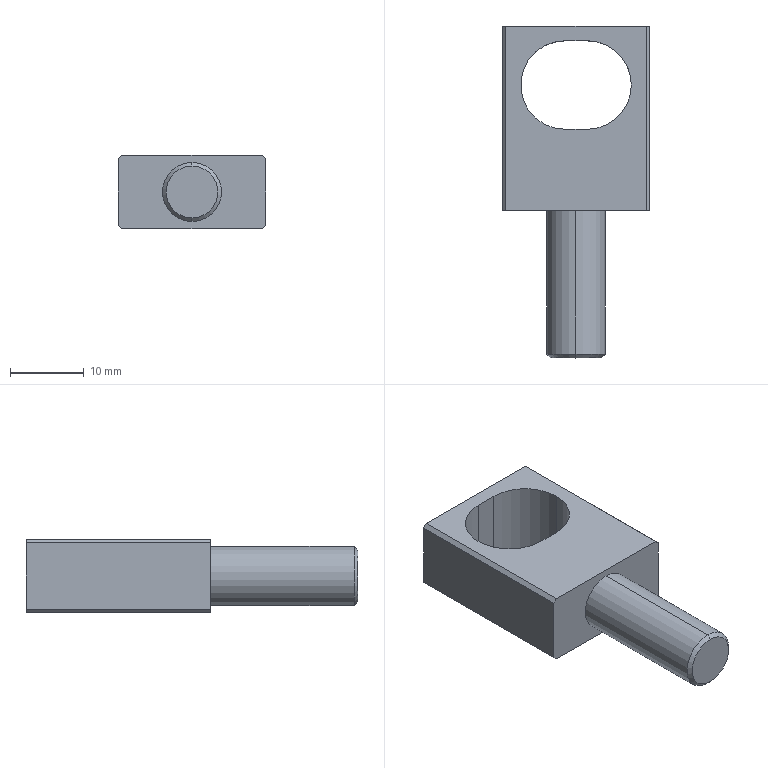Part | STEP file | 8ZY.143.1010 | 1 solid | 20 faces | box 20 x 45 x 10 mm | volume 4499 mm3 | plane 13 | cylinder 5 | cone 2 | commonest cylinder face diameters 12 x3 8 x2
STEP:
#1=CARTESIAN_POINT('',(0.,0.,0.));
#2=DIRECTION('',(0.,0.,1.));
#3=DIRECTION('',(1.,0.,0.));
#4=AXIS2_PLACEMENT_3D('',#1,#2,#3);
#5=CARTESIAN_POINT('',(1.5,10.5,-10.));
#6=VERTEX_POINT('',#5);
#7=CARTESIAN_POINT('',(1.5,10.5,0.));
#8=VERTEX_POINT('',#7);
#9=CARTESIAN_POINT('',(1.5,10.5,-10.));
#10=DIRECTION('',(0.,0.,1.));
#11=VECTOR('',#10,1.);
#12=LINE('',#9,#11);
#13=CARTESIAN_POINT('',(1.5,4.5,-10.));
#14=DIRECTION('',(0.,0.,1.));
#15=DIRECTION('',(1.,0.,0.));
#16=AXIS2_PLACEMENT_3D('',#13,#14,#15);
#17=CYLINDRICAL_SURFACE('',#16,6.);
#18=CARTESIAN_POINT('',(1.571,0.));
#19=DIRECTION('',(0.,1.));
#20=VECTOR('',#19,1.);
#21=LINE('',#18,#20);
#22=(GEOMETRIC_REPRESENTATION_CONTEXT(2)PARAMETRIC_REPRESENTATION_CONTEXT()REPRESENTATION_CONTEXT('',''));
#23=DEFINITIONAL_REPRESENTATION('',(#21),#22);
#24=PCURVE('',#17,#23);
#25=CARTESIAN_POINT('',(-1.5,10.5,-10.));
#26=DIRECTION('',(0.,1.,0.));
#27=DIRECTION('',(0.,0.,1.));
#28=AXIS2_PLACEMENT_3D('',#25,#26,#27);
#29=PLANE('',#28);
#30=CARTESIAN_POINT('',(0.,3.));
#31=DIRECTION('',(1.,0.));
#32=VECTOR('',#31,1.);
#33=LINE('',#30,#32);
#34=(GEOMETRIC_REPRESENTATION_CONTEXT(2)PARAMETRIC_REPRESENTATION_CONTEXT()REPRESENTATION_CONTEXT('',''));
#35=DEFINITIONAL_REPRESENTATION('',(#33),#34);
#36=PCURVE('',#29,#35);
#37=SURFACE_CURVE('',#12,(#24,#36),.PCURVE_S1.);
#38=EDGE_CURVE('',#6,#8,#37,.T.);
#39=ORIENTED_EDGE('',*,*,#38,.T.);
#40=CARTESIAN_POINT('',(7.5,4.5,0.));
#41=VERTEX_POINT('',#40);
#42=CARTESIAN_POINT('',(1.5,4.5,0.));
#43=DIRECTION('',(0.,0.,1.));
#44=DIRECTION('',(1.,0.,0.));
#45=AXIS2_PLACEMENT_3D('',#42,#43,#44);
#46=CIRCLE('',#45,6.);
#47=CARTESIAN_POINT('',(0.,10.));
#48=DIRECTION('',(1.,0.));
#49=VECTOR('',#48,1.);
#50=LINE('',#47,#49);
#51=(GEOMETRIC_REPRESENTATION_CONTEXT(2)PARAMETRIC_REPRESENTATION_CONTEXT()REPRESENTATION_CONTEXT('',''));
#52=DEFINITIONAL_REPRESENTATION('',(#50),#51);
#53=PCURVE('',#17,#52);
#54=CARTESIAN_POINT('',(-10.,-12.5,0.));
#55=DIRECTION('',(0.,0.,-1.));
#56=DIRECTION('',(-1.,0.,0.));
#57=AXIS2_PLACEMENT_3D('',#54,#55,#56);
#58=PLANE('',#57);
#59=CARTESIAN_POINT('',(-17.5,17.));
#60=CARTESIAN_POINT('',(-17.5,27.392));
#61=CARTESIAN_POINT('',(-8.5,22.196));
#62=CARTESIAN_POINT('',(0.5,17.));
#63=CARTESIAN_POINT('',(-8.5,11.804));
#64=CARTESIAN_POINT('',(-17.5,6.608));
#65=CARTESIAN_POINT('',(-17.5,17.));
#66=(BOUNDED_CURVE()B_SPLINE_CURVE(2,(#59,#60,#61,#62,#63,#64,#65),.UNSPECIFIED.,.T.,.F.)B_SPLINE_CURVE_WITH_KNOTS((1,2,2,2,2,1),(-2.094,0.,2.094,4.189,6.283,8.378),.UNSPECIFIED.)CURVE()GEOMETRIC_REPRESENTATION_ITEM()RATIONAL_B_SPLINE_CURVE((1.,0.5,1.,0.5,1.,0.5,1.))REPRESENTATION_ITEM(''));
#67=(GEOMETRIC_REPRESENTATION_CONTEXT(2)PARAMETRIC_REPRESENTATION_CONTEXT()REPRESENTATION_CONTEXT('',''));
#68=DEFINITIONAL_REPRESENTATION('',(#66),#67);
#69=PCURVE('',#58,#68);
#70=SURFACE_CURVE('',#46,(#53,#69),.PCURVE_S1.);
#71=EDGE_CURVE('',#41,#8,#70,.T.);
#72=ORIENTED_EDGE('',*,*,#71,.F.);
#73=CARTESIAN_POINT('',(7.5,4.5,-10.));
#74=VERTEX_POINT('',#73);
#75=CARTESIAN_POINT('',(7.5,4.5,-10.));
#76=DIRECTION('',(0.,0.,1.));
#77=VECTOR('',#76,1.);
#78=LINE('',#75,#77);
#79=CARTESIAN_POINT('',(0.,0.));
#80=DIRECTION('',(0.,1.));
#81=VECTOR('',#80,1.);
#82=LINE('',#79,#81);
#83=(GEOMETRIC_REPRESENTATION_CONTEXT(2)PARAMETRIC_REPRESENTATION_CONTEXT()REPRESENTATION_CONTEXT('',''));
#84=DEFINITIONAL_REPRESENTATION('',(#82),#83);
#85=PCURVE('',#17,#84);
#86=CARTESIAN_POINT('',(1.5,4.5,-10.));
#87=DIRECTION('',(0.,0.,1.));
#88=DIRECTION('',(1.,0.,0.));
#89=AXIS2_PLACEMENT_3D('',#86,#87,#88);
#90=CYLINDRICAL_SURFACE('',#89,6.);
#91=CARTESIAN_POINT('',(6.283,0.));
#92=DIRECTION('',(0.,1.));
#93=VECTOR('',#92,1.);
#94=LINE('',#91,#93);
#95=(GEOMETRIC_REPRESENTATION_CONTEXT(2)PARAMETRIC_REPRESENTATION_CONTEXT()REPRESENTATION_CONTEXT('',''));
#96=DEFINITIONAL_REPRESENTATION('',(#94),#95);
#97=PCURVE('',#90,#96);
#98=SURFACE_CURVE('',#78,(#85,#97),.PCURVE_S1.);
#99=EDGE_CURVE('',#74,#41,#98,.T.);
#100=ORIENTED_EDGE('',*,*,#99,.F.);
#101=CARTESIAN_POINT('',(1.5,4.5,-10.));
#102=DIRECTION('',(0.,0.,1.));
#103=DIRECTION('',(1.,0.,0.));
#104=AXIS2_PLACEMENT_3D('',#101,#102,#103);
#105=CIRCLE('',#104,6.);
#106=CARTESIAN_POINT('',(0.,0.));
#107=DIRECTION('',(1.,0.));
#108=VECTOR('',#107,1.);
#109=LINE('',#106,#108);
#110=(GEOMETRIC_REPRESENTATION_CONTEXT(2)PARAMETRIC_REPRESENTATION_CONTEXT()REPRESENTATION_CONTEXT('',''));
#111=DEFINITIONAL_REPRESENTATION('',(#109),#110);
#112=PCURVE('',#17,#111);
#113=CARTESIAN_POINT('',(-10.,-12.5,-10.));
#114=DIRECTION('',(0.,0.,-1.));
#115=DIRECTION('',(-1.,0.,0.));
#116=AXIS2_PLACEMENT_3D('',#113,#114,#115);
#117=PLANE('',#116);
#118=CARTESIAN_POINT('',(-17.5,17.));
#119=CARTESIAN_POINT('',(-17.5,27.392));
#120=CARTESIAN_POINT('',(-8.5,22.196));
#121=CARTESIAN_POINT('',(0.5,17.));
#122=CARTESIAN_POINT('',(-8.5,11.804));
#123=CARTESIAN_POINT('',(-17.5,6.608));
#124=CARTESIAN_POINT('',(-17.5,17.));
#125=(BOUNDED_CURVE()B_SPLINE_CURVE(2,(#118,#119,#120,#121,#122,#123,#124),.UNSPECIFIED.,.T.,.F.)B_SPLINE_CURVE_WITH_KNOTS((1,2,2,2,2,1),(-2.094,0.,2.094,4.189,6.283,8.378),.UNSPECIFIED.)CURVE()GEOMETRIC_REPRESENTATION_ITEM()RATIONAL_B_SPLINE_CURVE((1.,0.5,1.,0.5,1.,0.5,1.))REPRESENTATION_ITEM(''));
#126=(GEOMETRIC_REPRESENTATION_CONTEXT(2)PARAMETRIC_REPRESENTATION_CONTEXT()REPRESENTATION_CONTEXT('',''));
#127=DEFINITIONAL_REPRESENTATION('',(#125),#126);
#128=PCURVE('',#117,#127);
#129=SURFACE_CURVE('',#105,(#112,#128),.PCURVE_S1.);
#130=EDGE_CURVE('',#74,#6,#129,.T.);
#131=ORIENTED_EDGE('',*,*,#130,.T.);
#132=EDGE_LOOP('',(#39,#72,#100,#131));
#133=FACE_BOUND('',#132,.F.);
#134=ADVANCED_FACE('',(#133),#17,.F.);
#135=CARTESIAN_POINT('',(0.,-32.5,-8.5));
#136=VERTEX_POINT('',#135);
#137=CARTESIAN_POINT('',(0.,-32.5,-1.5));
#138=VERTEX_POINT('',#137);
#139=CARTESIAN_POINT('',(0.,-32.5,-5.));
#140=DIRECTION('',(0.,-1.,0.));
#141=DIRECTION('',(0.,0.,-1.));
#142=AXIS2_PLACEMENT_3D('',#139,#140,#141);
#143=CIRCLE('',#142,3.5);
#144=CARTESIAN_POINT('',(0.,-32.5,-5.));
#145=DIRECTION('',(0.,1.,0.));
#146=DIRECTION('',(0.,0.,1.));
#147=AXIS2_PLACEMENT_3D('',#144,#145,#146);
#148=CONICAL_SURFACE('',#147,3.5,0.7854);
#149=CARTESIAN_POINT('',(3.142,0.));
#150=DIRECTION('',(-1.,0.));
#151=VECTOR('',#150,1.);
#152=LINE('',#149,#151);
#153=(GEOMETRIC_REPRESENTATION_CONTEXT(2)PARAMETRIC_REPRESENTATION_CONTEXT()REPRESENTATION_CONTEXT('',''));
#154=DEFINITIONAL_REPRESENTATION('',(#152),#153);
#155=PCURVE('',#148,#154);
#156=CARTESIAN_POINT('',(0.,-32.5,-5.));
#157=DIRECTION('',(0.,-1.,0.));
#158=DIRECTION('',(0.,0.,-1.));
#159=AXIS2_PLACEMENT_3D('',#156,#157,#158);
#160=PLANE('',#159);
#161=CARTESIAN_POINT('',(0.,0.));
#162=DIRECTION('',(1.,0.));
#163=AXIS2_PLACEMENT_2D('',#161,#162);
#164=CIRCLE('',#163,3.5);
#165=(GEOMETRIC_REPRESENTATION_CONTEXT(2)PARAMETRIC_REPRESENTATION_CONTEXT()REPRESENTATION_CONTEXT('',''));
#166=DEFINITIONAL_REPRESENTATION('',(#164),#165);
#167=PCURVE('',#160,#166);
#168=SURFACE_CURVE('',#143,(#155,#167),.PCURVE_S1.);
#169=EDGE_CURVE('',#136,#138,#168,.T.);
#170=ORIENTED_EDGE('',*,*,#169,.F.);
#171=CARTESIAN_POINT('',(0.,-32.,-9.));
#172=VERTEX_POINT('',#171);
#173=CARTESIAN_POINT('',(0.,-32.5,-8.5));
#174=DIRECTION('',(0.,0.7071,-0.7071));
#175=VECTOR('',#174,1.);
#176=LINE('',#173,#175);
#177=CARTESIAN_POINT('',(3.142,0.));
#178=DIRECTION('',(0.,1.));
#179=VECTOR('',#178,1.);
#180=LINE('',#177,#179);
#181=(GEOMETRIC_REPRESENTATION_CONTEXT(2)PARAMETRIC_REPRESENTATION_CONTEXT()REPRESENTATION_CONTEXT('',''));
#182=DEFINITIONAL_REPRESENTATION('',(#180),#181);
#183=PCURVE('',#148,#182);
#184=CARTESIAN_POINT('',(0.,-32.5,-5.));
#185=DIRECTION('',(0.,1.,0.));
#186=DIRECTION('',(0.,0.,1.));
#187=AXIS2_PLACEMENT_3D('',#184,#185,#186);
#188=CONICAL_SURFACE('',#187,3.5,0.7854);
#189=CARTESIAN_POINT('',(3.142,0.));
#190=DIRECTION('',(0.,1.));
#191=VECTOR('',#190,1.);
#192=LINE('',#189,#191);
#193=(GEOMETRIC_REPRESENTATION_CONTEXT(2)PARAMETRIC_REPRESENTATION_CONTEXT()REPRESENTATION_CONTEXT('',''));
#194=DEFINITIONAL_REPRESENTATION('',(#192),#193);
#195=PCURVE('',#188,#194);
#196=SURFACE_CURVE('',#176,(#183,#195),.PCURVE_S1.);
#197=EDGE_CURVE('',#136,#172,#196,.T.);
#198=ORIENTED_EDGE('',*,*,#197,.T.);
#199=CARTESIAN_POINT('',(0.,-32.,-1.));
#200=VERTEX_POINT('',#199);
#201=CARTESIAN_POINT('',(0.,-32.,-5.));
#202=DIRECTION('',(0.,1.,0.));
#203=DIRECTION('',(0.,0.,-1.));
#204=AXIS2_PLACEMENT_3D('',#201,#202,#203);
#205=CIRCLE('',#204,4.);
#206=CARTESIAN_POINT('',(-3.142,0.5));
#207=DIRECTION('',(1.,0.));
#208=VECTOR('',#207,1.);
#209=LINE('',#206,#208);
#210=(GEOMETRIC_REPRESENTATION_CONTEXT(2)PARAMETRIC_REPRESENTATION_CONTEXT()REPRESENTATION_CONTEXT('',''));
#211=DEFINITIONAL_REPRESENTATION('',(#209),#210);
#212=PCURVE('',#148,#211);
#213=CARTESIAN_POINT('',(0.,-32.5,-5.));
#214=DIRECTION('',(0.,1.,0.));
#215=DIRECTION('',(0.,0.,1.));
#216=AXIS2_PLACEMENT_3D('',#213,#214,#215);
#217=CYLINDRICAL_SURFACE('',#216,4.);
#218=CARTESIAN_POINT('',(-3.142,0.5));
#219=DIRECTION('',(1.,0.));
#220=VECTOR('',#219,1.);
#221=LINE('',#218,#220);
#222=(GEOMETRIC_REPRESENTATION_CONTEXT(2)PARAMETRIC_REPRESENTATION_CONTEXT()REPRESENTATION_CONTEXT('',''));
#223=DEFINITIONAL_REPRESENTATION('',(#221),#222);
#224=PCURVE('',#217,#223);
#225=SURFACE_CURVE('',#205,(#212,#224),.PCURVE_S1.);
#226=EDGE_CURVE('',#200,#172,#225,.T.);
#227=ORIENTED_EDGE('',*,*,#226,.F.);
#228=CARTESIAN_POINT('',(0.,-32.5,-1.5));
#229=DIRECTION('',(0.,0.7071,0.7071));
#230=VECTOR('',#229,1.);
#231=LINE('',#228,#230);
#232=CARTESIAN_POINT('',(0.,0.));
#233=DIRECTION('',(0.,1.));
#234=VECTOR('',#233,1.);
#235=LINE('',#232,#234);
#236=(GEOMETRIC_REPRESENTATION_CONTEXT(2)PARAMETRIC_REPRESENTATION_CONTEXT()REPRESENTATION_CONTEXT('',''));
#237=DEFINITIONAL_REPRESENTATION('',(#235),#236);
#238=PCURVE('',#148,#237);
#239=CARTESIAN_POINT('',(6.283,0.));
#240=DIRECTION('',(0.,1.));
#241=VECTOR('',#240,1.);
#242=LINE('',#239,#241);
#243=(GEOMETRIC_REPRESENTATION_CONTEXT(2)PARAMETRIC_REPRESENTATION_CONTEXT()REPRESENTATION_CONTEXT('',''));
#244=DEFINITIONAL_REPRESENTATION('',(#242),#243);
#245=PCURVE('',#188,#244);
#246=SURFACE_CURVE('',#231,(#238,#245),.PCURVE_S1.);
#247=EDGE_CURVE('',#138,#200,#246,.T.);
#248=ORIENTED_EDGE('',*,*,#247,.F.);
#249=EDGE_LOOP('',(#170,#198,#227,#248));
#250=FACE_BOUND('',#249,.T.);
#251=ADVANCED_FACE('',(#250),#148,.T.);
#252=ORIENTED_EDGE('',*,*,#226,.T.);
#253=CARTESIAN_POINT('',(0.,-12.5,-9.));
#254=VERTEX_POINT('',#253);
#255=CARTESIAN_POINT('',(0.,-32.5,-9.));
#256=DIRECTION('',(0.,1.,0.));
#257=VECTOR('',#256,1.);
#258=LINE('',#255,#257);
#259=CARTESIAN_POINT('',(3.142,0.));
#260=DIRECTION('',(0.,1.));
#261=VECTOR('',#260,1.);
#262=LINE('',#259,#261);
#263=(GEOMETRIC_REPRESENTATION_CONTEXT(2)PARAMETRIC_REPRESENTATION_CONTEXT()REPRESENTATION_CONTEXT('',''));
#264=DEFINITIONAL_REPRESENTATION('',(#262),#263);
#265=PCURVE('',#217,#264);
#266=CARTESIAN_POINT('',(0.,-32.5,-5.));
#267=DIRECTION('',(0.,1.,0.));
#268=DIRECTION('',(0.,0.,1.));
#269=AXIS2_PLACEMENT_3D('',#266,#267,#268);
#270=CYLINDRICAL_SURFACE('',#269,4.);
#271=CARTESIAN_POINT('',(3.142,0.));
#272=DIRECTION('',(0.,1.));
#273=VECTOR('',#272,1.);
#274=LINE('',#271,#273);
#275=(GEOMETRIC_REPRESENTATION_CONTEXT(2)PARAMETRIC_REPRESENTATION_CONTEXT()REPRESENTATION_CONTEXT('',''));
#276=DEFINITIONAL_REPRESENTATION('',(#274),#275);
#277=PCURVE('',#270,#276);
#278=SURFACE_CURVE('',#258,(#265,#277),.PCURVE_S1.);
#279=EDGE_CURVE('',#172,#254,#278,.T.);
#280=ORIENTED_EDGE('',*,*,#279,.T.);
#281=CARTESIAN_POINT('',(0.,-12.5,-1.));
#282=VERTEX_POINT('',#281);
#283=CARTESIAN_POINT('',(0.,-12.5,-5.));
#284=DIRECTION('',(0.,-1.,0.));
#285=DIRECTION('',(0.,0.,-1.));
#286=AXIS2_PLACEMENT_3D('',#283,#284,#285);
#287=CIRCLE('',#286,4.);
#288=CARTESIAN_POINT('',(3.142,20.));
#289=DIRECTION('',(-1.,0.));
#290=VECTOR('',#289,1.);
#291=LINE('',#288,#290);
#292=(GEOMETRIC_REPRESENTATION_CONTEXT(2)PARAMETRIC_REPRESENTATION_CONTEXT()REPRESENTATION_CONTEXT('',''));
#293=DEFINITIONAL_REPRESENTATION('',(#291),#292);
#294=PCURVE('',#217,#293);
#295=CARTESIAN_POINT('',(10.,-12.5,-10.));
#296=DIRECTION('',(0.,-1.,0.));
#297=DIRECTION('',(1.,0.,0.));
#298=AXIS2_PLACEMENT_3D('',#295,#296,#297);
#299=PLANE('',#298);
#300=CARTESIAN_POINT('',(-10.,5.));
#301=DIRECTION('',(0.,-1.));
#302=AXIS2_PLACEMENT_2D('',#300,#301);
#303=CIRCLE('',#302,4.);
#304=(GEOMETRIC_REPRESENTATION_CONTEXT(2)PARAMETRIC_REPRESENTATION_CONTEXT()REPRESENTATION_CONTEXT('',''));
#305=DEFINITIONAL_REPRESENTATION('',(#303),#304);
#306=PCURVE('',#299,#305);
#307=SURFACE_CURVE('',#287,(#294,#306),.PCURVE_S1.);
#308=EDGE_CURVE('',#254,#282,#307,.T.);
#309=ORIENTED_EDGE('',*,*,#308,.T.);
#310=CARTESIAN_POINT('',(0.,-32.5,-1.));
#311=DIRECTION('',(0.,1.,0.));
#312=VECTOR('',#311,1.);
#313=LINE('',#310,#312);
#314=CARTESIAN_POINT('',(0.,0.));
#315=DIRECTION('',(0.,1.));
#316=VECTOR('',#315,1.);
#317=LINE('',#314,#316);
#318=(GEOMETRIC_REPRESENTATION_CONTEXT(2)PARAMETRIC_REPRESENTATION_CONTEXT()REPRESENTATION_CONTEXT('',''));
#319=DEFINITIONAL_REPRESENTATION('',(#317),#318);
#320=PCURVE('',#217,#319);
#321=CARTESIAN_POINT('',(6.283,0.));
#322=DIRECTION('',(0.,1.));
#323=VECTOR('',#322,1.);
#324=LINE('',#321,#323);
#325=(GEOMETRIC_REPRESENTATION_CONTEXT(2)PARAMETRIC_REPRESENTATION_CONTEXT()REPRESENTATION_CONTEXT('',''));
#326=DEFINITIONAL_REPRESENTATION('',(#324),#325);
#327=PCURVE('',#270,#326);
#328=SURFACE_CURVE('',#313,(#320,#327),.PCURVE_S1.);
#329=EDGE_CURVE('',#200,#282,#328,.T.);
#330=ORIENTED_EDGE('',*,*,#329,.F.);
#331=EDGE_LOOP('',(#252,#280,#309,#330));
#332=FACE_BOUND('',#331,.T.);
#333=ADVANCED_FACE('',(#332),#217,.T.);
#334=CARTESIAN_POINT('',(-9.5,-12.5,0.));
#335=VERTEX_POINT('',#334);
#336=CARTESIAN_POINT('',(9.5,-12.5,0.));
#337=VERTEX_POINT('',#336);
#338=CARTESIAN_POINT('',(10.,-12.5,0.));
#339=DIRECTION('',(1.,0.,0.));
#340=VECTOR('',#339,1.);
#341=LINE('',#338,#340);
#342=CARTESIAN_POINT('',(0.,10.));
#343=DIRECTION('',(1.,0.));
#344=VECTOR('',#343,1.);
#345=LINE('',#342,#344);
#346=(GEOMETRIC_REPRESENTATION_CONTEXT(2)PARAMETRIC_REPRESENTATION_CONTEXT()REPRESENTATION_CONTEXT('',''));
#347=DEFINITIONAL_REPRESENTATION('',(#345),#346);
#348=PCURVE('',#299,#347);
#349=CARTESIAN_POINT('',(-20.,0.));
#350=DIRECTION('',(-1.,0.));
#351=VECTOR('',#350,1.);
#352=LINE('',#349,#351);
#353=(GEOMETRIC_REPRESENTATION_CONTEXT(2)PARAMETRIC_REPRESENTATION_CONTEXT()REPRESENTATION_CONTEXT('',''));
#354=DEFINITIONAL_REPRESENTATION('',(#352),#353);
#355=PCURVE('',#58,#354);
#356=SURFACE_CURVE('',#341,(#348,#355),.PCURVE_S1.);
#357=EDGE_CURVE('',#335,#337,#356,.T.);
#358=ORIENTED_EDGE('',*,*,#357,.F.);
#359=CARTESIAN_POINT('',(-10.,-12.5,-0.5));
#360=VERTEX_POINT('',#359);
#361=CARTESIAN_POINT('',(-4.75,-12.5,4.75));
#362=DIRECTION('',(-0.7071,0.,-0.7071));
#363=VECTOR('',#362,1.);
#364=LINE('',#361,#363);
#365=CARTESIAN_POINT('',(-14.75,14.75));
#366=DIRECTION('',(-0.7071,-0.7071));
#367=VECTOR('',#366,1.);
#368=LINE('',#365,#367);
#369=(GEOMETRIC_REPRESENTATION_CONTEXT(2)PARAMETRIC_REPRESENTATION_CONTEXT()REPRESENTATION_CONTEXT('',''));
#370=DEFINITIONAL_REPRESENTATION('',(#368),#369);
#371=PCURVE('',#299,#370);
#372=CARTESIAN_POINT('',(-9.5,-12.5,0.));
#373=DIRECTION('',(-0.7071,0.,0.7071));
#374=DIRECTION('',(0.7071,0.,0.7071));
#375=AXIS2_PLACEMENT_3D('',#372,#373,#374);
#376=PLANE('',#375);
#377=CARTESIAN_POINT('',(6.718,0.));
#378=DIRECTION('',(-1.,0.));
#379=VECTOR('',#378,1.);
#380=LINE('',#377,#379);
#381=(GEOMETRIC_REPRESENTATION_CONTEXT(2)PARAMETRIC_REPRESENTATION_CONTEXT()REPRESENTATION_CONTEXT('',''));
#382=DEFINITIONAL_REPRESENTATION('',(#380),#381);
#383=PCURVE('',#376,#382);
#384=SURFACE_CURVE('',#364,(#371,#383),.PCURVE_S1.);
#385=EDGE_CURVE('',#335,#360,#384,.T.);
#386=ORIENTED_EDGE('',*,*,#385,.T.);
#387=CARTESIAN_POINT('',(-10.,-12.5,-9.5));
#388=VERTEX_POINT('',#387);
#389=CARTESIAN_POINT('',(-10.,-12.5,-10.));
#390=DIRECTION('',(0.,0.,1.));
#391=VECTOR('',#390,1.);
#392=LINE('',#389,#391);
#393=CARTESIAN_POINT('',(-20.,0.));
#394=DIRECTION('',(0.,1.));
#395=VECTOR('',#394,1.);
#396=LINE('',#393,#395);
#397=(GEOMETRIC_REPRESENTATION_CONTEXT(2)PARAMETRIC_REPRESENTATION_CONTEXT()REPRESENTATION_CONTEXT('',''));
#398=DEFINITIONAL_REPRESENTATION('',(#396),#397);
#399=PCURVE('',#299,#398);
#400=CARTESIAN_POINT('',(-10.,12.5,-10.));
#401=DIRECTION('',(-1.,0.,0.));
#402=DIRECTION('',(0.,-1.,0.));
#403=AXIS2_PLACEMENT_3D('',#400,#401,#402);
#404=PLANE('',#403);
#405=CARTESIAN_POINT('',(25.,0.));
#406=DIRECTION('',(0.,1.));
#407=VECTOR('',#406,1.);
#408=LINE('',#405,#407);
#409=(GEOMETRIC_REPRESENTATION_CONTEXT(2)PARAMETRIC_REPRESENTATION_CONTEXT()REPRESENTATION_CONTEXT('',''));
#410=DEFINITIONAL_REPRESENTATION('',(#408),#409);
#411=PCURVE('',#404,#410);
#412=SURFACE_CURVE('',#392,(#399,#411),.PCURVE_S1.);
#413=EDGE_CURVE('',#388,#360,#412,.T.);
#414=ORIENTED_EDGE('',*,*,#413,.F.);
#415=CARTESIAN_POINT('',(-9.5,-12.5,-10.));
#416=VERTEX_POINT('',#415);
#417=CARTESIAN_POINT('',(0.25,-12.5,-19.75));
#418=DIRECTION('',(0.7071,0.,-0.7071));
#419=VECTOR('',#418,1.);
#420=LINE('',#417,#419);
#421=CARTESIAN_POINT('',(-9.75,-9.75));
#422=DIRECTION('',(0.7071,-0.7071));
#423=VECTOR('',#422,1.);
#424=LINE('',#421,#423);
#425=(GEOMETRIC_REPRESENTATION_CONTEXT(2)PARAMETRIC_REPRESENTATION_CONTEXT()REPRESENTATION_CONTEXT('',''));
#426=DEFINITIONAL_REPRESENTATION('',(#424),#425);
#427=PCURVE('',#299,#426);
#428=CARTESIAN_POINT('',(-10.,12.5,-9.5));
#429=DIRECTION('',(0.7071,0.,0.7071));
#430=DIRECTION('',(0.7071,0.,-0.7071));
#431=AXIS2_PLACEMENT_3D('',#428,#429,#430);
#432=PLANE('',#431);
#433=CARTESIAN_POINT('',(14.496,-25.));
#434=DIRECTION('',(1.,0.));
#435=VECTOR('',#434,1.);
#436=LINE('',#433,#435);
#437=(GEOMETRIC_REPRESENTATION_CONTEXT(2)PARAMETRIC_REPRESENTATION_CONTEXT()REPRESENTATION_CONTEXT('',''));
#438=DEFINITIONAL_REPRESENTATION('',(#436),#437);
#439=PCURVE('',#432,#438);
#440=SURFACE_CURVE('',#420,(#427,#439),.PCURVE_S1.);
#441=EDGE_CURVE('',#388,#416,#440,.T.);
#442=ORIENTED_EDGE('',*,*,#441,.T.);
#443=CARTESIAN_POINT('',(9.5,-12.5,-10.));
#444=VERTEX_POINT('',#443);
#445=CARTESIAN_POINT('',(10.,-12.5,-10.));
#446=DIRECTION('',(1.,0.,0.));
#447=VECTOR('',#446,1.);
#448=LINE('',#445,#447);
#449=CARTESIAN_POINT('',(0.,0.));
#450=DIRECTION('',(1.,0.));
#451=VECTOR('',#450,1.);
#452=LINE('',#449,#451);
#453=(GEOMETRIC_REPRESENTATION_CONTEXT(2)PARAMETRIC_REPRESENTATION_CONTEXT()REPRESENTATION_CONTEXT('',''));
#454=DEFINITIONAL_REPRESENTATION('',(#452),#453);
#455=PCURVE('',#299,#454);
#456=CARTESIAN_POINT('',(-20.,0.));
#457=DIRECTION('',(-1.,0.));
#458=VECTOR('',#457,1.);
#459=LINE('',#456,#458);
#460=(GEOMETRIC_REPRESENTATION_CONTEXT(2)PARAMETRIC_REPRESENTATION_CONTEXT()REPRESENTATION_CONTEXT('',''));
#461=DEFINITIONAL_REPRESENTATION('',(#459),#460);
#462=PCURVE('',#117,#461);
#463=SURFACE_CURVE('',#448,(#455,#462),.PCURVE_S1.);
#464=EDGE_CURVE('',#416,#444,#463,.T.);
#465=ORIENTED_EDGE('',*,*,#464,.T.);
#466=CARTESIAN_POINT('',(10.,-12.5,-9.5));
#467=VERTEX_POINT('',#466);
#468=CARTESIAN_POINT('',(9.75,-12.5,-9.75));
#469=DIRECTION('',(0.7071,0.,0.7071));
#470=VECTOR('',#469,1.);
#471=LINE('',#468,#470);
#472=CARTESIAN_POINT('',(-0.25,0.25));
#473=DIRECTION('',(0.7071,0.7071));
#474=VECTOR('',#473,1.);
#475=LINE('',#472,#474);
#476=(GEOMETRIC_REPRESENTATION_CONTEXT(2)PARAMETRIC_REPRESENTATION_CONTEXT()REPRESENTATION_CONTEXT('',''));
#477=DEFINITIONAL_REPRESENTATION('',(#475),#476);
#478=PCURVE('',#299,#477);
#479=CARTESIAN_POINT('',(10.,12.5,-9.5));
#480=DIRECTION('',(-0.7071,0.,0.7071));
#481=DIRECTION('',(0.7071,0.,0.7071));
#482=AXIS2_PLACEMENT_3D('',#479,#480,#481);
#483=PLANE('',#482);
#484=CARTESIAN_POINT('',(-0.3536,-25.));
#485=DIRECTION('',(1.,0.));
#486=VECTOR('',#485,1.);
#487=LINE('',#484,#486);
#488=(GEOMETRIC_REPRESENTATION_CONTEXT(2)PARAMETRIC_REPRESENTATION_CONTEXT()REPRESENTATION_CONTEXT('',''));
#489=DEFINITIONAL_REPRESENTATION('',(#487),#488);
#490=PCURVE('',#483,#489);
#491=SURFACE_CURVE('',#471,(#478,#490),.PCURVE_S1.);
#492=EDGE_CURVE('',#444,#467,#491,.T.);
#493=ORIENTED_EDGE('',*,*,#492,.T.);
#494=CARTESIAN_POINT('',(10.,-12.5,-0.5));
#495=VERTEX_POINT('',#494);
#496=CARTESIAN_POINT('',(10.,-12.5,-10.));
#497=DIRECTION('',(0.,0.,1.));
#498=VECTOR('',#497,1.);
#499=LINE('',#496,#498);
#500=CARTESIAN_POINT('',(0.,0.));
#501=DIRECTION('',(0.,1.));
#502=VECTOR('',#501,1.);
#503=LINE('',#500,#502);
#504=(GEOMETRIC_REPRESENTATION_CONTEXT(2)PARAMETRIC_REPRESENTATION_CONTEXT()REPRESENTATION_CONTEXT('',''));
#505=DEFINITIONAL_REPRESENTATION('',(#503),#504);
#506=PCURVE('',#299,#505);
#507=CARTESIAN_POINT('',(10.,12.5,-10.));
#508=DIRECTION('',(1.,0.,0.));
#509=DIRECTION('',(0.,1.,0.));
#510=AXIS2_PLACEMENT_3D('',#507,#508,#509);
#511=PLANE('',#510);
#512=CARTESIAN_POINT('',(-25.,0.));
#513=DIRECTION('',(0.,1.));
#514=VECTOR('',#513,1.);
#515=LINE('',#512,#514);
#516=(GEOMETRIC_REPRESENTATION_CONTEXT(2)PARAMETRIC_REPRESENTATION_CONTEXT()REPRESENTATION_CONTEXT('',''));
#517=DEFINITIONAL_REPRESENTATION('',(#515),#516);
#518=PCURVE('',#511,#517);
#519=SURFACE_CURVE('',#499,(#506,#518),.PCURVE_S1.);
#520=EDGE_CURVE('',#467,#495,#519,.T.);
#521=ORIENTED_EDGE('',*,*,#520,.T.);
#522=CARTESIAN_POINT('',(14.75,-12.5,-5.25));
#523=DIRECTION('',(-0.7071,0.,0.7071));
#524=VECTOR('',#523,1.);
#525=LINE('',#522,#524);
#526=CARTESIAN_POINT('',(4.75,4.75));
#527=DIRECTION('',(-0.7071,0.7071));
#528=VECTOR('',#527,1.);
#529=LINE('',#526,#528);
#530=(GEOMETRIC_REPRESENTATION_CONTEXT(2)PARAMETRIC_REPRESENTATION_CONTEXT()REPRESENTATION_CONTEXT('',''));
#531=DEFINITIONAL_REPRESENTATION('',(#529),#530);
#532=PCURVE('',#299,#531);
#533=CARTESIAN_POINT('',(9.5,-12.5,0.));
#534=DIRECTION('',(0.7071,0.,0.7071));
#535=DIRECTION('',(0.7071,0.,-0.7071));
#536=AXIS2_PLACEMENT_3D('',#533,#534,#535);
#537=PLANE('',#536);
#538=CARTESIAN_POINT('',(7.425,0.));
#539=DIRECTION('',(-1.,0.));
#540=VECTOR('',#539,1.);
#541=LINE('',#538,#540);
#542=(GEOMETRIC_REPRESENTATION_CONTEXT(2)PARAMETRIC_REPRESENTATION_CONTEXT()REPRESENTATION_CONTEXT('',''));
#543=DEFINITIONAL_REPRESENTATION('',(#541),#542);
#544=PCURVE('',#537,#543);
#545=SURFACE_CURVE('',#525,(#532,#544),.PCURVE_S1.);
#546=EDGE_CURVE('',#495,#337,#545,.T.);
#547=ORIENTED_EDGE('',*,*,#546,.T.);
#548=EDGE_LOOP('',(#358,#386,#414,#442,#465,#493,#521,#547));
#549=FACE_BOUND('',#548,.T.);
#550=CARTESIAN_POINT('',(0.,-12.5,-5.));
#551=DIRECTION('',(0.,-1.,0.));
#552=DIRECTION('',(0.,0.,-1.));
#553=AXIS2_PLACEMENT_3D('',#550,#551,#552);
#554=CIRCLE('',#553,4.);
#555=CARTESIAN_POINT('',(-10.,5.));
#556=DIRECTION('',(0.,-1.));
#557=AXIS2_PLACEMENT_2D('',#555,#556);
#558=CIRCLE('',#557,4.);
#559=(GEOMETRIC_REPRESENTATION_CONTEXT(2)PARAMETRIC_REPRESENTATION_CONTEXT()REPRESENTATION_CONTEXT('',''));
#560=DEFINITIONAL_REPRESENTATION('',(#558),#559);
#561=PCURVE('',#299,#560);
#562=CARTESIAN_POINT('',(9.425,20.));
#563=DIRECTION('',(-1.,0.));
#564=VECTOR('',#563,1.);
#565=LINE('',#562,#564);
#566=(GEOMETRIC_REPRESENTATION_CONTEXT(2)PARAMETRIC_REPRESENTATION_CONTEXT()REPRESENTATION_CONTEXT('',''));
#567=DEFINITIONAL_REPRESENTATION('',(#565),#566);
#568=PCURVE('',#270,#567);
#569=SURFACE_CURVE('',#554,(#561,#568),.PCURVE_S1.);
#570=EDGE_CURVE('',#282,#254,#569,.T.);
#571=ORIENTED_EDGE('',*,*,#570,.F.);
#572=ORIENTED_EDGE('',*,*,#308,.F.);
#573=EDGE_LOOP('',(#571,#572));
#574=FACE_BOUND('',#573,.T.);
#575=ADVANCED_FACE('',(#549,#574),#299,.T.);
#576=ORIENTED_EDGE('',*,*,#413,.T.);
#577=CARTESIAN_POINT('',(-10.,12.5,-0.5));
#578=VERTEX_POINT('',#577);
#579=CARTESIAN_POINT('',(-10.,12.5,-0.5));
#580=DIRECTION('',(0.,1.,0.));
#581=VECTOR('',#580,1.);
#582=LINE('',#579,#581);
#583=CARTESIAN_POINT('',(0.,9.5));
#584=DIRECTION('',(-1.,0.));
#585=VECTOR('',#584,1.);
#586=LINE('',#583,#585);
#587=(GEOMETRIC_REPRESENTATION_CONTEXT(2)PARAMETRIC_REPRESENTATION_CONTEXT()REPRESENTATION_CONTEXT('',''));
#588=DEFINITIONAL_REPRESENTATION('',(#586),#587);
#589=PCURVE('',#404,#588);
#590=CARTESIAN_POINT('',(-0.7071,25.));
#591=DIRECTION('',(0.,1.));
#592=VECTOR('',#591,1.);
#593=LINE('',#590,#592);
#594=(GEOMETRIC_REPRESENTATION_CONTEXT(2)PARAMETRIC_REPRESENTATION_CONTEXT()REPRESENTATION_CONTEXT('',''));
#595=DEFINITIONAL_REPRESENTATION('',(#593),#594);
#596=PCURVE('',#376,#595);
#597=SURFACE_CURVE('',#582,(#589,#596),.PCURVE_S1.);
#598=EDGE_CURVE('',#360,#578,#597,.T.);
#599=ORIENTED_EDGE('',*,*,#598,.T.);
#600=CARTESIAN_POINT('',(-10.,12.5,-9.5));
#601=VERTEX_POINT('',#600);
#602=CARTESIAN_POINT('',(-10.,12.5,-10.));
#603=DIRECTION('',(0.,0.,1.));
#604=VECTOR('',#603,1.);
#605=LINE('',#602,#604);
#606=CARTESIAN_POINT('',(0.,0.));
#607=DIRECTION('',(0.,1.));
#608=VECTOR('',#607,1.);
#609=LINE('',#606,#608);
#610=(GEOMETRIC_REPRESENTATION_CONTEXT(2)PARAMETRIC_REPRESENTATION_CONTEXT()REPRESENTATION_CONTEXT('',''));
#611=DEFINITIONAL_REPRESENTATION('',(#609),#610);
#612=PCURVE('',#404,#611);
#613=CARTESIAN_POINT('',(10.,12.5,-10.));
#614=DIRECTION('',(0.,1.,0.));
#615=DIRECTION('',(-1.,0.,0.));
#616=AXIS2_PLACEMENT_3D('',#613,#614,#615);
#617=PLANE('',#616);
#618=CARTESIAN_POINT('',(20.,0.));
#619=DIRECTION('',(0.,1.));
#620=VECTOR('',#619,1.);
#621=LINE('',#618,#620);
#622=(GEOMETRIC_REPRESENTATION_CONTEXT(2)PARAMETRIC_REPRESENTATION_CONTEXT()REPRESENTATION_CONTEXT('',''));
#623=DEFINITIONAL_REPRESENTATION('',(#621),#622);
#624=PCURVE('',#617,#623);
#625=SURFACE_CURVE('',#605,(#612,#624),.PCURVE_S1.);
#626=EDGE_CURVE('',#601,#578,#625,.T.);
#627=ORIENTED_EDGE('',*,*,#626,.F.);
#628=CARTESIAN_POINT('',(-10.,12.5,-9.5));
#629=DIRECTION('',(0.,-1.,0.));
#630=VECTOR('',#629,1.);
#631=LINE('',#628,#630);
#632=CARTESIAN_POINT('',(0.,0.5));
#633=DIRECTION('',(1.,0.));
#634=VECTOR('',#633,1.);
#635=LINE('',#632,#634);
#636=(GEOMETRIC_REPRESENTATION_CONTEXT(2)PARAMETRIC_REPRESENTATION_CONTEXT()REPRESENTATION_CONTEXT('',''));
#637=DEFINITIONAL_REPRESENTATION('',(#635),#636);
#638=PCURVE('',#404,#637);
#639=CARTESIAN_POINT('',(0.,0.));
#640=DIRECTION('',(0.,-1.));
#641=VECTOR('',#640,1.);
#642=LINE('',#639,#641);
#643=(GEOMETRIC_REPRESENTATION_CONTEXT(2)PARAMETRIC_REPRESENTATION_CONTEXT()REPRESENTATION_CONTEXT('',''));
#644=DEFINITIONAL_REPRESENTATION('',(#642),#643);
#645=PCURVE('',#432,#644);
#646=SURFACE_CURVE('',#631,(#638,#645),.PCURVE_S1.);
#647=EDGE_CURVE('',#601,#388,#646,.T.);
#648=ORIENTED_EDGE('',*,*,#647,.T.);
#649=EDGE_LOOP('',(#576,#599,#627,#648));
#650=FACE_BOUND('',#649,.T.);
#651=ADVANCED_FACE('',(#650),#404,.T.);
#652=ORIENTED_EDGE('',*,*,#626,.T.);
#653=CARTESIAN_POINT('',(-9.5,12.5,0.));
#654=VERTEX_POINT('',#653);
#655=CARTESIAN_POINT('',(-4.75,12.5,4.75));
#656=DIRECTION('',(0.7071,0.,0.7071));
#657=VECTOR('',#656,1.);
#658=LINE('',#655,#657);
#659=CARTESIAN_POINT('',(14.75,14.75));
#660=DIRECTION('',(-0.7071,0.7071));
#661=VECTOR('',#660,1.);
#662=LINE('',#659,#661);
#663=(GEOMETRIC_REPRESENTATION_CONTEXT(2)PARAMETRIC_REPRESENTATION_CONTEXT()REPRESENTATION_CONTEXT('',''));
#664=DEFINITIONAL_REPRESENTATION('',(#662),#663);
#665=PCURVE('',#617,#664);
#666=CARTESIAN_POINT('',(6.718,25.));
#667=DIRECTION('',(1.,0.));
#668=VECTOR('',#667,1.);
#669=LINE('',#666,#668);
#670=(GEOMETRIC_REPRESENTATION_CONTEXT(2)PARAMETRIC_REPRESENTATION_CONTEXT()REPRESENTATION_CONTEXT('',''));
#671=DEFINITIONAL_REPRESENTATION('',(#669),#670);
#672=PCURVE('',#376,#671);
#673=SURFACE_CURVE('',#658,(#665,#672),.PCURVE_S1.);
#674=EDGE_CURVE('',#578,#654,#673,.T.);
#675=ORIENTED_EDGE('',*,*,#674,.T.);
#676=CARTESIAN_POINT('',(9.5,12.5,0.));
#677=VERTEX_POINT('',#676);
#678=CARTESIAN_POINT('',(10.,12.5,0.));
#679=DIRECTION('',(-1.,0.,0.));
#680=VECTOR('',#679,1.);
#681=LINE('',#678,#680);
#682=CARTESIAN_POINT('',(0.,10.));
#683=DIRECTION('',(1.,0.));
#684=VECTOR('',#683,1.);
#685=LINE('',#682,#684);
#686=(GEOMETRIC_REPRESENTATION_CONTEXT(2)PARAMETRIC_REPRESENTATION_CONTEXT()REPRESENTATION_CONTEXT('',''));
#687=DEFINITIONAL_REPRESENTATION('',(#685),#686);
#688=PCURVE('',#617,#687);
#689=CARTESIAN_POINT('',(-20.,25.));
#690=DIRECTION('',(1.,0.));
#691=VECTOR('',#690,1.);
#692=LINE('',#689,#691);
#693=(GEOMETRIC_REPRESENTATION_CONTEXT(2)PARAMETRIC_REPRESENTATION_CONTEXT()REPRESENTATION_CONTEXT('',''));
#694=DEFINITIONAL_REPRESENTATION('',(#692),#693);
#695=PCURVE('',#58,#694);
#696=SURFACE_CURVE('',#681,(#688,#695),.PCURVE_S1.);
#697=EDGE_CURVE('',#677,#654,#696,.T.);
#698=ORIENTED_EDGE('',*,*,#697,.F.);
#699=CARTESIAN_POINT('',(10.,12.5,-0.5));
#700=VERTEX_POINT('',#699);
#701=CARTESIAN_POINT('',(14.75,12.5,-5.25));
#702=DIRECTION('',(0.7071,0.,-0.7071));
#703=VECTOR('',#702,1.);
#704=LINE('',#701,#703);
#705=CARTESIAN_POINT('',(-4.75,4.75));
#706=DIRECTION('',(-0.7071,-0.7071));
#707=VECTOR('',#706,1.);
#708=LINE('',#705,#707);
#709=(GEOMETRIC_REPRESENTATION_CONTEXT(2)PARAMETRIC_REPRESENTATION_CONTEXT()REPRESENTATION_CONTEXT('',''));
#710=DEFINITIONAL_REPRESENTATION('',(#708),#709);
#711=PCURVE('',#617,#710);
#712=CARTESIAN_POINT('',(7.425,25.));
#713=DIRECTION('',(1.,0.));
#714=VECTOR('',#713,1.);
#715=LINE('',#712,#714);
#716=(GEOMETRIC_REPRESENTATION_CONTEXT(2)PARAMETRIC_REPRESENTATION_CONTEXT()REPRESENTATION_CONTEXT('',''));
#717=DEFINITIONAL_REPRESENTATION('',(#715),#716);
#718=PCURVE('',#537,#717);
#719=SURFACE_CURVE('',#704,(#711,#718),.PCURVE_S1.);
#720=EDGE_CURVE('',#677,#700,#719,.T.);
#721=ORIENTED_EDGE('',*,*,#720,.T.);
#722=CARTESIAN_POINT('',(10.,12.5,-9.5));
#723=VERTEX_POINT('',#722);
#724=CARTESIAN_POINT('',(10.,12.5,-10.));
#725=DIRECTION('',(0.,0.,1.));
#726=VECTOR('',#725,1.);
#727=LINE('',#724,#726);
#728=CARTESIAN_POINT('',(0.,0.));
#729=DIRECTION('',(0.,1.));
#730=VECTOR('',#729,1.);
#731=LINE('',#728,#730);
#732=(GEOMETRIC_REPRESENTATION_CONTEXT(2)PARAMETRIC_REPRESENTATION_CONTEXT()REPRESENTATION_CONTEXT('',''));
#733=DEFINITIONAL_REPRESENTATION('',(#731),#732);
#734=PCURVE('',#617,#733);
#735=CARTESIAN_POINT('',(0.,0.));
#736=DIRECTION('',(0.,1.));
#737=VECTOR('',#736,1.);
#738=LINE('',#735,#737);
#739=(GEOMETRIC_REPRESENTATION_CONTEXT(2)PARAMETRIC_REPRESENTATION_CONTEXT()REPRESENTATION_CONTEXT('',''));
#740=DEFINITIONAL_REPRESENTATION('',(#738),#739);
#741=PCURVE('',#511,#740);
#742=SURFACE_CURVE('',#727,(#734,#741),.PCURVE_S1.);
#743=EDGE_CURVE('',#723,#700,#742,.T.);
#744=ORIENTED_EDGE('',*,*,#743,.F.);
#745=CARTESIAN_POINT('',(9.5,12.5,-10.));
#746=VERTEX_POINT('',#745);
#747=CARTESIAN_POINT('',(9.75,12.5,-9.75));
#748=DIRECTION('',(-0.7071,0.,-0.7071));
#749=VECTOR('',#748,1.);
#750=LINE('',#747,#749);
#751=CARTESIAN_POINT('',(0.25,0.25));
#752=DIRECTION('',(0.7071,-0.7071));
#753=VECTOR('',#752,1.);
#754=LINE('',#751,#753);
#755=(GEOMETRIC_REPRESENTATION_CONTEXT(2)PARAMETRIC_REPRESENTATION_CONTEXT()REPRESENTATION_CONTEXT('',''));
#756=DEFINITIONAL_REPRESENTATION('',(#754),#755);
#757=PCURVE('',#617,#756);
#758=CARTESIAN_POINT('',(-0.3536,0.));
#759=DIRECTION('',(-1.,0.));
#760=VECTOR('',#759,1.);
#761=LINE('',#758,#760);
#762=(GEOMETRIC_REPRESENTATION_CONTEXT(2)PARAMETRIC_REPRESENTATION_CONTEXT()REPRESENTATION_CONTEXT('',''));
#763=DEFINITIONAL_REPRESENTATION('',(#761),#762);
#764=PCURVE('',#483,#763);
#765=SURFACE_CURVE('',#750,(#757,#764),.PCURVE_S1.);
#766=EDGE_CURVE('',#723,#746,#765,.T.);
#767=ORIENTED_EDGE('',*,*,#766,.T.);
#768=CARTESIAN_POINT('',(-9.5,12.5,-10.));
#769=VERTEX_POINT('',#768);
#770=CARTESIAN_POINT('',(10.,12.5,-10.));
#771=DIRECTION('',(-1.,0.,0.));
#772=VECTOR('',#771,1.);
#773=LINE('',#770,#772);
#774=CARTESIAN_POINT('',(0.,0.));
#775=DIRECTION('',(1.,0.));
#776=VECTOR('',#775,1.);
#777=LINE('',#774,#776);
#778=(GEOMETRIC_REPRESENTATION_CONTEXT(2)PARAMETRIC_REPRESENTATION_CONTEXT()REPRESENTATION_CONTEXT('',''));
#779=DEFINITIONAL_REPRESENTATION('',(#777),#778);
#780=PCURVE('',#617,#779);
#781=CARTESIAN_POINT('',(-20.,25.));
#782=DIRECTION('',(1.,0.));
#783=VECTOR('',#782,1.);
#784=LINE('',#781,#783);
#785=(GEOMETRIC_REPRESENTATION_CONTEXT(2)PARAMETRIC_REPRESENTATION_CONTEXT()REPRESENTATION_CONTEXT('',''));
#786=DEFINITIONAL_REPRESENTATION('',(#784),#785);
#787=PCURVE('',#117,#786);
#788=SURFACE_CURVE('',#773,(#780,#787),.PCURVE_S1.);
#789=EDGE_CURVE('',#746,#769,#788,.T.);
#790=ORIENTED_EDGE('',*,*,#789,.T.);
#791=CARTESIAN_POINT('',(0.25,12.5,-19.75));
#792=DIRECTION('',(-0.7071,0.,0.7071));
#793=VECTOR('',#792,1.);
#794=LINE('',#791,#793);
#795=CARTESIAN_POINT('',(9.75,-9.75));
#796=DIRECTION('',(0.7071,0.7071));
#797=VECTOR('',#796,1.);
#798=LINE('',#795,#797);
#799=(GEOMETRIC_REPRESENTATION_CONTEXT(2)PARAMETRIC_REPRESENTATION_CONTEXT()REPRESENTATION_CONTEXT('',''));
#800=DEFINITIONAL_REPRESENTATION('',(#798),#799);
#801=PCURVE('',#617,#800);
#802=CARTESIAN_POINT('',(14.496,0.));
#803=DIRECTION('',(-1.,0.));
#804=VECTOR('',#803,1.);
#805=LINE('',#802,#804);
#806=(GEOMETRIC_REPRESENTATION_CONTEXT(2)PARAMETRIC_REPRESENTATION_CONTEXT()REPRESENTATION_CONTEXT('',''));
#807=DEFINITIONAL_REPRESENTATION('',(#805),#806);
#808=PCURVE('',#432,#807);
#809=SURFACE_CURVE('',#794,(#801,#808),.PCURVE_S1.);
#810=EDGE_CURVE('',#769,#601,#809,.T.);
#811=ORIENTED_EDGE('',*,*,#810,.T.);
#812=EDGE_LOOP('',(#652,#675,#698,#721,#744,#767,#790,#811));
#813=FACE_BOUND('',#812,.T.);
#814=ADVANCED_FACE('',(#813),#617,.T.);
#815=ORIENTED_EDGE('',*,*,#520,.F.);
#816=CARTESIAN_POINT('',(10.,12.5,-9.5));
#817=DIRECTION('',(0.,1.,0.));
#818=VECTOR('',#817,1.);
#819=LINE('',#816,#818);
#820=CARTESIAN_POINT('',(0.,0.5));
#821=DIRECTION('',(1.,0.));
#822=VECTOR('',#821,1.);
#823=LINE('',#820,#822);
#824=(GEOMETRIC_REPRESENTATION_CONTEXT(2)PARAMETRIC_REPRESENTATION_CONTEXT()REPRESENTATION_CONTEXT('',''));
#825=DEFINITIONAL_REPRESENTATION('',(#823),#824);
#826=PCURVE('',#511,#825);
#827=CARTESIAN_POINT('',(0.,0.));
#828=DIRECTION('',(0.,1.));
#829=VECTOR('',#828,1.);
#830=LINE('',#827,#829);
#831=(GEOMETRIC_REPRESENTATION_CONTEXT(2)PARAMETRIC_REPRESENTATION_CONTEXT()REPRESENTATION_CONTEXT('',''));
#832=DEFINITIONAL_REPRESENTATION('',(#830),#831);
#833=PCURVE('',#483,#832);
#834=SURFACE_CURVE('',#819,(#826,#833),.PCURVE_S1.);
#835=EDGE_CURVE('',#467,#723,#834,.T.);
#836=ORIENTED_EDGE('',*,*,#835,.T.);
#837=ORIENTED_EDGE('',*,*,#743,.T.);
#838=CARTESIAN_POINT('',(10.,-12.5,-0.5));
#839=DIRECTION('',(0.,-1.,0.));
#840=VECTOR('',#839,1.);
#841=LINE('',#838,#840);
#842=CARTESIAN_POINT('',(-25.,9.5));
#843=DIRECTION('',(-1.,0.));
#844=VECTOR('',#843,1.);
#845=LINE('',#842,#844);
#846=(GEOMETRIC_REPRESENTATION_CONTEXT(2)PARAMETRIC_REPRESENTATION_CONTEXT()REPRESENTATION_CONTEXT('',''));
#847=DEFINITIONAL_REPRESENTATION('',(#845),#846);
#848=PCURVE('',#511,#847);
#849=CARTESIAN_POINT('',(0.7071,0.));
#850=DIRECTION('',(0.,-1.));
#851=VECTOR('',#850,1.);
#852=LINE('',#849,#851);
#853=(GEOMETRIC_REPRESENTATION_CONTEXT(2)PARAMETRIC_REPRESENTATION_CONTEXT()REPRESENTATION_CONTEXT('',''));
#854=DEFINITIONAL_REPRESENTATION('',(#852),#853);
#855=PCURVE('',#537,#854);
#856=SURFACE_CURVE('',#841,(#848,#855),.PCURVE_S1.);
#857=EDGE_CURVE('',#700,#495,#856,.T.);
#858=ORIENTED_EDGE('',*,*,#857,.T.);
#859=EDGE_LOOP('',(#815,#836,#837,#858));
#860=FACE_BOUND('',#859,.T.);
#861=ADVANCED_FACE('',(#860),#511,.T.);
#862=CARTESIAN_POINT('',(-1.5,10.5,-10.));
#863=VERTEX_POINT('',#862);
#864=CARTESIAN_POINT('',(-1.5,-1.5,-10.));
#865=VERTEX_POINT('',#864);
#866=CARTESIAN_POINT('',(-1.5,4.5,-10.));
#867=DIRECTION('',(0.,0.,1.));
#868=DIRECTION('',(1.,0.,0.));
#869=AXIS2_PLACEMENT_3D('',#866,#867,#868);
#870=CIRCLE('',#869,6.);
#871=CARTESIAN_POINT('',(-14.5,17.));
#872=CARTESIAN_POINT('',(-14.5,27.392));
#873=CARTESIAN_POINT('',(-5.5,22.196));
#874=CARTESIAN_POINT('',(3.5,17.));
#875=CARTESIAN_POINT('',(-5.5,11.804));
#876=CARTESIAN_POINT('',(-14.5,6.608));
#877=CARTESIAN_POINT('',(-14.5,17.));
#878=(BOUNDED_CURVE()B_SPLINE_CURVE(2,(#871,#872,#873,#874,#875,#876,#877),.UNSPECIFIED.,.T.,.F.)B_SPLINE_CURVE_WITH_KNOTS((1,2,2,2,2,1),(-2.094,0.,2.094,4.189,6.283,8.378),.UNSPECIFIED.)CURVE()GEOMETRIC_REPRESENTATION_ITEM()RATIONAL_B_SPLINE_CURVE((1.,0.5,1.,0.5,1.,0.5,1.))REPRESENTATION_ITEM(''));
#879=(GEOMETRIC_REPRESENTATION_CONTEXT(2)PARAMETRIC_REPRESENTATION_CONTEXT()REPRESENTATION_CONTEXT('',''));
#880=DEFINITIONAL_REPRESENTATION('',(#878),#879);
#881=PCURVE('',#117,#880);
#882=CARTESIAN_POINT('',(-1.5,4.5,-10.));
#883=DIRECTION('',(0.,0.,1.));
#884=DIRECTION('',(1.,0.,0.));
#885=AXIS2_PLACEMENT_3D('',#882,#883,#884);
#886=CYLINDRICAL_SURFACE('',#885,6.);
#887=CARTESIAN_POINT('',(0.,0.));
#888=DIRECTION('',(1.,0.));
#889=VECTOR('',#888,1.);
#890=LINE('',#887,#889);
#891=(GEOMETRIC_REPRESENTATION_CONTEXT(2)PARAMETRIC_REPRESENTATION_CONTEXT()REPRESENTATION_CONTEXT('',''));
#892=DEFINITIONAL_REPRESENTATION('',(#890),#891);
#893=PCURVE('',#886,#892);
#894=SURFACE_CURVE('',#870,(#881,#893),.PCURVE_S1.);
#895=EDGE_CURVE('',#863,#865,#894,.T.);
#896=ORIENTED_EDGE('',*,*,#895,.T.);
#897=CARTESIAN_POINT('',(1.5,-1.5,-10.));
#898=VERTEX_POINT('',#897);
#899=CARTESIAN_POINT('',(-1.5,-1.5,-10.));
#900=DIRECTION('',(1.,0.,0.));
#901=VECTOR('',#900,1.);
#902=LINE('',#899,#901);
#903=CARTESIAN_POINT('',(-8.5,11.));
#904=DIRECTION('',(-1.,0.));
#905=VECTOR('',#904,1.);
#906=LINE('',#903,#905);
#907=(GEOMETRIC_REPRESENTATION_CONTEXT(2)PARAMETRIC_REPRESENTATION_CONTEXT()REPRESENTATION_CONTEXT('',''));
#908=DEFINITIONAL_REPRESENTATION('',(#906),#907);
#909=PCURVE('',#117,#908);
#910=CARTESIAN_POINT('',(-1.5,-1.5,-10.));
#911=DIRECTION('',(0.,-1.,0.));
#912=DIRECTION('',(1.,0.,0.));
#913=AXIS2_PLACEMENT_3D('',#910,#911,#912);
#914=PLANE('',#913);
#915=CARTESIAN_POINT('',(0.,0.));
#916=DIRECTION('',(1.,0.));
#917=VECTOR('',#916,1.);
#918=LINE('',#915,#917);
#919=(GEOMETRIC_REPRESENTATION_CONTEXT(2)PARAMETRIC_REPRESENTATION_CONTEXT()REPRESENTATION_CONTEXT('',''));
#920=DEFINITIONAL_REPRESENTATION('',(#918),#919);
#921=PCURVE('',#914,#920);
#922=SURFACE_CURVE('',#902,(#909,#921),.PCURVE_S1.);
#923=EDGE_CURVE('',#865,#898,#922,.T.);
#924=ORIENTED_EDGE('',*,*,#923,.T.);
#925=CARTESIAN_POINT('',(1.5,4.5,-10.));
#926=DIRECTION('',(0.,0.,1.));
#927=DIRECTION('',(1.,0.,0.));
#928=AXIS2_PLACEMENT_3D('',#925,#926,#927);
#929=CIRCLE('',#928,6.);
#930=CARTESIAN_POINT('',(-17.5,17.));
#931=CARTESIAN_POINT('',(-17.5,27.392));
#932=CARTESIAN_POINT('',(-8.5,22.196));
#933=CARTESIAN_POINT('',(0.5,17.));
#934=CARTESIAN_POINT('',(-8.5,11.804));
#935=CARTESIAN_POINT('',(-17.5,6.608));
#936=CARTESIAN_POINT('',(-17.5,17.));
#937=(BOUNDED_CURVE()B_SPLINE_CURVE(2,(#930,#931,#932,#933,#934,#935,#936),.UNSPECIFIED.,.T.,.F.)B_SPLINE_CURVE_WITH_KNOTS((1,2,2,2,2,1),(-2.094,0.,2.094,4.189,6.283,8.378),.UNSPECIFIED.)CURVE()GEOMETRIC_REPRESENTATION_ITEM()RATIONAL_B_SPLINE_CURVE((1.,0.5,1.,0.5,1.,0.5,1.))REPRESENTATION_ITEM(''));
#938=(GEOMETRIC_REPRESENTATION_CONTEXT(2)PARAMETRIC_REPRESENTATION_CONTEXT()REPRESENTATION_CONTEXT('',''));
#939=DEFINITIONAL_REPRESENTATION('',(#937),#938);
#940=PCURVE('',#117,#939);
#941=CARTESIAN_POINT('',(0.,0.));
#942=DIRECTION('',(1.,0.));
#943=VECTOR('',#942,1.);
#944=LINE('',#941,#943);
#945=(GEOMETRIC_REPRESENTATION_CONTEXT(2)PARAMETRIC_REPRESENTATION_CONTEXT()REPRESENTATION_CONTEXT('',''));
#946=DEFINITIONAL_REPRESENTATION('',(#944),#945);
#947=PCURVE('',#90,#946);
#948=SURFACE_CURVE('',#929,(#940,#947),.PCURVE_S1.);
#949=EDGE_CURVE('',#898,#74,#948,.T.);
#950=ORIENTED_EDGE('',*,*,#949,.T.);
#951=ORIENTED_EDGE('',*,*,#130,.T.);
#952=CARTESIAN_POINT('',(-1.5,10.5,-10.));
#953=DIRECTION('',(-1.,0.,0.));
#954=VECTOR('',#953,1.);
#955=LINE('',#952,#954);
#956=CARTESIAN_POINT('',(-8.5,23.));
#957=DIRECTION('',(1.,0.));
#958=VECTOR('',#957,1.);
#959=LINE('',#956,#958);
#960=(GEOMETRIC_REPRESENTATION_CONTEXT(2)PARAMETRIC_REPRESENTATION_CONTEXT()REPRESENTATION_CONTEXT('',''));
#961=DEFINITIONAL_REPRESENTATION('',(#959),#960);
#962=PCURVE('',#117,#961);
#963=CARTESIAN_POINT('',(0.,0.));
#964=DIRECTION('',(0.,-1.));
#965=VECTOR('',#964,1.);
#966=LINE('',#963,#965);
#967=(GEOMETRIC_REPRESENTATION_CONTEXT(2)PARAMETRIC_REPRESENTATION_CONTEXT()REPRESENTATION_CONTEXT('',''));
#968=DEFINITIONAL_REPRESENTATION('',(#966),#967);
#969=PCURVE('',#29,#968);
#970=SURFACE_CURVE('',#955,(#962,#969),.PCURVE_S1.);
#971=EDGE_CURVE('',#6,#863,#970,.T.);
#972=ORIENTED_EDGE('',*,*,#971,.T.);
#973=EDGE_LOOP('',(#896,#924,#950,#951,#972));
#974=FACE_BOUND('',#973,.T.);
#975=ORIENTED_EDGE('',*,*,#464,.F.);
#976=CARTESIAN_POINT('',(-9.5,-12.5,-10.));
#977=DIRECTION('',(0.,1.,0.));
#978=VECTOR('',#977,1.);
#979=LINE('',#976,#978);
#980=CARTESIAN_POINT('',(-0.5,0.));
#981=DIRECTION('',(0.,1.));
#982=VECTOR('',#981,1.);
#983=LINE('',#980,#982);
#984=(GEOMETRIC_REPRESENTATION_CONTEXT(2)PARAMETRIC_REPRESENTATION_CONTEXT()REPRESENTATION_CONTEXT('',''));
#985=DEFINITIONAL_REPRESENTATION('',(#983),#984);
#986=PCURVE('',#117,#985);
#987=CARTESIAN_POINT('',(0.7071,-25.));
#988=DIRECTION('',(0.,1.));
#989=VECTOR('',#988,1.);
#990=LINE('',#987,#989);
#991=(GEOMETRIC_REPRESENTATION_CONTEXT(2)PARAMETRIC_REPRESENTATION_CONTEXT()REPRESENTATION_CONTEXT('',''));
#992=DEFINITIONAL_REPRESENTATION('',(#990),#991);
#993=PCURVE('',#432,#992);
#994=SURFACE_CURVE('',#979,(#986,#993),.PCURVE_S1.);
#995=EDGE_CURVE('',#416,#769,#994,.T.);
#996=ORIENTED_EDGE('',*,*,#995,.T.);
#997=ORIENTED_EDGE('',*,*,#789,.F.);
#998=CARTESIAN_POINT('',(9.5,-12.5,-10.));
#999=DIRECTION('',(0.,-1.,0.));
#1000=VECTOR('',#999,1.);
#1001=LINE('',#998,#1000);
#1002=CARTESIAN_POINT('',(-19.5,0.));
#1003=DIRECTION('',(0.,-1.));
#1004=VECTOR('',#1003,1.);
#1005=LINE('',#1002,#1004);
#1006=(GEOMETRIC_REPRESENTATION_CONTEXT(2)PARAMETRIC_REPRESENTATION_CONTEXT()REPRESENTATION_CONTEXT('',''));
#1007=DEFINITIONAL_REPRESENTATION('',(#1005),#1006);
#1008=PCURVE('',#117,#1007);
#1009=CARTESIAN_POINT('',(-0.7071,-25.));
#1010=DIRECTION('',(0.,-1.));
#1011=VECTOR('',#1010,1.);
#1012=LINE('',#1009,#1011);
#1013=(GEOMETRIC_REPRESENTATION_CONTEXT(2)PARAMETRIC_REPRESENTATION_CONTEXT()REPRESENTATION_CONTEXT('',''));
#1014=DEFINITIONAL_REPRESENTATION('',(#1012),#1013);
#1015=PCURVE('',#483,#1014);
#1016=SURFACE_CURVE('',#1001,(#1008,#1015),.PCURVE_S1.);
#1017=EDGE_CURVE('',#746,#444,#1016,.T.);
#1018=ORIENTED_EDGE('',*,*,#1017,.T.);
#1019=EDGE_LOOP('',(#975,#996,#997,#1018));
#1020=FACE_BOUND('',#1019,.T.);
#1021=ADVANCED_FACE('',(#974,#1020),#117,.T.);
#1022=CARTESIAN_POINT('',(-1.5,-1.5,0.));
#1023=VERTEX_POINT('',#1022);
#1024=CARTESIAN_POINT('',(1.5,-1.5,0.));
#1025=VERTEX_POINT('',#1024);
#1026=CARTESIAN_POINT('',(-1.5,-1.5,0.));
#1027=DIRECTION('',(1.,0.,0.));
#1028=VECTOR('',#1027,1.);
#1029=LINE('',#1026,#1028);
#1030=CARTESIAN_POINT('',(-8.5,11.));
#1031=DIRECTION('',(-1.,0.));
#1032=VECTOR('',#1031,1.);
#1033=LINE('',#1030,#1032);
#1034=(GEOMETRIC_REPRESENTATION_CONTEXT(2)PARAMETRIC_REPRESENTATION_CONTEXT()REPRESENTATION_CONTEXT('',''));
#1035=DEFINITIONAL_REPRESENTATION('',(#1033),#1034);
#1036=PCURVE('',#58,#1035);
#1037=CARTESIAN_POINT('',(0.,10.));
#1038=DIRECTION('',(1.,0.));
#1039=VECTOR('',#1038,1.);
#1040=LINE('',#1037,#1039);
#1041=(GEOMETRIC_REPRESENTATION_CONTEXT(2)PARAMETRIC_REPRESENTATION_CONTEXT()REPRESENTATION_CONTEXT('',''));
#1042=DEFINITIONAL_REPRESENTATION('',(#1040),#1041);
#1043=PCURVE('',#914,#1042);
#1044=SURFACE_CURVE('',#1029,(#1036,#1043),.PCURVE_S1.);
#1045=EDGE_CURVE('',#1023,#1025,#1044,.T.);
#1046=ORIENTED_EDGE('',*,*,#1045,.F.);
#1047=CARTESIAN_POINT('',(-1.5,10.5,0.));
#1048=VERTEX_POINT('',#1047);
#1049=CARTESIAN_POINT('',(-1.5,4.5,0.));
#1050=DIRECTION('',(0.,0.,1.));
#1051=DIRECTION('',(1.,0.,0.));
#1052=AXIS2_PLACEMENT_3D('',#1049,#1050,#1051);
#1053=CIRCLE('',#1052,6.);
#1054=CARTESIAN_POINT('',(-14.5,17.));
#1055=CARTESIAN_POINT('',(-14.5,27.392));
#1056=CARTESIAN_POINT('',(-5.5,22.196));
#1057=CARTESIAN_POINT('',(3.5,17.));
#1058=CARTESIAN_POINT('',(-5.5,11.804));
#1059=CARTESIAN_POINT('',(-14.5,6.608));
#1060=CARTESIAN_POINT('',(-14.5,17.));
#1061=(BOUNDED_CURVE()B_SPLINE_CURVE(2,(#1054,#1055,#1056,#1057,#1058,#1059,#1060),.UNSPECIFIED.,.T.,.F.)B_SPLINE_CURVE_WITH_KNOTS((1,2,2,2,2,1),(-2.094,0.,2.094,4.189,6.283,8.378),.UNSPECIFIED.)CURVE()GEOMETRIC_REPRESENTATION_ITEM()RATIONAL_B_SPLINE_CURVE((1.,0.5,1.,0.5,1.,0.5,1.))REPRESENTATION_ITEM(''));
#1062=(GEOMETRIC_REPRESENTATION_CONTEXT(2)PARAMETRIC_REPRESENTATION_CONTEXT()REPRESENTATION_CONTEXT('',''));
#1063=DEFINITIONAL_REPRESENTATION('',(#1061),#1062);
#1064=PCURVE('',#58,#1063);
#1065=CARTESIAN_POINT('',(0.,10.));
#1066=DIRECTION('',(1.,0.));
#1067=VECTOR('',#1066,1.);
#1068=LINE('',#1065,#1067);
#1069=(GEOMETRIC_REPRESENTATION_CONTEXT(2)PARAMETRIC_REPRESENTATION_CONTEXT()REPRESENTATION_CONTEXT('',''));
#1070=DEFINITIONAL_REPRESENTATION('',(#1068),#1069);
#1071=PCURVE('',#886,#1070);
#1072=SURFACE_CURVE('',#1053,(#1064,#1071),.PCURVE_S1.);
#1073=EDGE_CURVE('',#1048,#1023,#1072,.T.);
#1074=ORIENTED_EDGE('',*,*,#1073,.F.);
#1075=CARTESIAN_POINT('',(-1.5,10.5,0.));
#1076=DIRECTION('',(-1.,0.,0.));
#1077=VECTOR('',#1076,1.);
#1078=LINE('',#1075,#1077);
#1079=CARTESIAN_POINT('',(-8.5,23.));
#1080=DIRECTION('',(1.,0.));
#1081=VECTOR('',#1080,1.);
#1082=LINE('',#1079,#1081);
#1083=(GEOMETRIC_REPRESENTATION_CONTEXT(2)PARAMETRIC_REPRESENTATION_CONTEXT()REPRESENTATION_CONTEXT('',''));
#1084=DEFINITIONAL_REPRESENTATION('',(#1082),#1083);
#1085=PCURVE('',#58,#1084);
#1086=CARTESIAN_POINT('',(10.,0.));
#1087=DIRECTION('',(0.,-1.));
#1088=VECTOR('',#1087,1.);
#1089=LINE('',#1086,#1088);
#1090=(GEOMETRIC_REPRESENTATION_CONTEXT(2)PARAMETRIC_REPRESENTATION_CONTEXT()REPRESENTATION_CONTEXT('',''));
#1091=DEFINITIONAL_REPRESENTATION('',(#1089),#1090);
#1092=PCURVE('',#29,#1091);
#1093=SURFACE_CURVE('',#1078,(#1085,#1092),.PCURVE_S1.);
#1094=EDGE_CURVE('',#8,#1048,#1093,.T.);
#1095=ORIENTED_EDGE('',*,*,#1094,.F.);
#1096=ORIENTED_EDGE('',*,*,#71,.F.);
#1097=CARTESIAN_POINT('',(1.5,4.5,0.));
#1098=DIRECTION('',(0.,0.,1.));
#1099=DIRECTION('',(1.,0.,0.));
#1100=AXIS2_PLACEMENT_3D('',#1097,#1098,#1099);
#1101=CIRCLE('',#1100,6.);
#1102=CARTESIAN_POINT('',(-17.5,17.));
#1103=CARTESIAN_POINT('',(-17.5,27.392));
#1104=CARTESIAN_POINT('',(-8.5,22.196));
#1105=CARTESIAN_POINT('',(0.5,17.));
#1106=CARTESIAN_POINT('',(-8.5,11.804));
#1107=CARTESIAN_POINT('',(-17.5,6.608));
#1108=CARTESIAN_POINT('',(-17.5,17.));
#1109=(BOUNDED_CURVE()B_SPLINE_CURVE(2,(#1102,#1103,#1104,#1105,#1106,#1107,#1108),.UNSPECIFIED.,.T.,.F.)B_SPLINE_CURVE_WITH_KNOTS((1,2,2,2,2,1),(-2.094,0.,2.094,4.189,6.283,8.378),.UNSPECIFIED.)CURVE()GEOMETRIC_REPRESENTATION_ITEM()RATIONAL_B_SPLINE_CURVE((1.,0.5,1.,0.5,1.,0.5,1.))REPRESENTATION_ITEM(''));
#1110=(GEOMETRIC_REPRESENTATION_CONTEXT(2)PARAMETRIC_REPRESENTATION_CONTEXT()REPRESENTATION_CONTEXT('',''));
#1111=DEFINITIONAL_REPRESENTATION('',(#1109),#1110);
#1112=PCURVE('',#58,#1111);
#1113=CARTESIAN_POINT('',(0.,10.));
#1114=DIRECTION('',(1.,0.));
#1115=VECTOR('',#1114,1.);
#1116=LINE('',#1113,#1115);
#1117=(GEOMETRIC_REPRESENTATION_CONTEXT(2)PARAMETRIC_REPRESENTATION_CONTEXT()REPRESENTATION_CONTEXT('',''));
#1118=DEFINITIONAL_REPRESENTATION('',(#1116),#1117);
#1119=PCURVE('',#90,#1118);
#1120=SURFACE_CURVE('',#1101,(#1112,#1119),.PCURVE_S1.);
#1121=EDGE_CURVE('',#1025,#41,#1120,.T.);
#1122=ORIENTED_EDGE('',*,*,#1121,.F.);
#1123=EDGE_LOOP('',(#1046,#1074,#1095,#1096,#1122));
#1124=FACE_BOUND('',#1123,.T.);
#1125=ORIENTED_EDGE('',*,*,#697,.T.);
#1126=CARTESIAN_POINT('',(-9.5,-12.5,0.));
#1127=DIRECTION('',(0.,-1.,0.));
#1128=VECTOR('',#1127,1.);
#1129=LINE('',#1126,#1128);
#1130=CARTESIAN_POINT('',(-0.5,0.));
#1131=DIRECTION('',(0.,-1.));
#1132=VECTOR('',#1131,1.);
#1133=LINE('',#1130,#1132);
#1134=(GEOMETRIC_REPRESENTATION_CONTEXT(2)PARAMETRIC_REPRESENTATION_CONTEXT()REPRESENTATION_CONTEXT('',''));
#1135=DEFINITIONAL_REPRESENTATION('',(#1133),#1134);
#1136=PCURVE('',#58,#1135);
#1137=CARTESIAN_POINT('',(0.,0.));
#1138=DIRECTION('',(0.,-1.));
#1139=VECTOR('',#1138,1.);
#1140=LINE('',#1137,#1139);
#1141=(GEOMETRIC_REPRESENTATION_CONTEXT(2)PARAMETRIC_REPRESENTATION_CONTEXT()REPRESENTATION_CONTEXT('',''));
#1142=DEFINITIONAL_REPRESENTATION('',(#1140),#1141);
#1143=PCURVE('',#376,#1142);
#1144=SURFACE_CURVE('',#1129,(#1136,#1143),.PCURVE_S1.);
#1145=EDGE_CURVE('',#654,#335,#1144,.T.);
#1146=ORIENTED_EDGE('',*,*,#1145,.T.);
#1147=ORIENTED_EDGE('',*,*,#357,.T.);
#1148=CARTESIAN_POINT('',(9.5,12.5,0.));
#1149=DIRECTION('',(0.,1.,0.));
#1150=VECTOR('',#1149,1.);
#1151=LINE('',#1148,#1150);
#1152=CARTESIAN_POINT('',(-19.5,25.));
#1153=DIRECTION('',(0.,1.));
#1154=VECTOR('',#1153,1.);
#1155=LINE('',#1152,#1154);
#1156=(GEOMETRIC_REPRESENTATION_CONTEXT(2)PARAMETRIC_REPRESENTATION_CONTEXT()REPRESENTATION_CONTEXT('',''));
#1157=DEFINITIONAL_REPRESENTATION('',(#1155),#1156);
#1158=PCURVE('',#58,#1157);
#1159=CARTESIAN_POINT('',(0.,25.));
#1160=DIRECTION('',(0.,1.));
#1161=VECTOR('',#1160,1.);
#1162=LINE('',#1159,#1161);
#1163=(GEOMETRIC_REPRESENTATION_CONTEXT(2)PARAMETRIC_REPRESENTATION_CONTEXT()REPRESENTATION_CONTEXT('',''));
#1164=DEFINITIONAL_REPRESENTATION('',(#1162),#1163);
#1165=PCURVE('',#537,#1164);
#1166=SURFACE_CURVE('',#1151,(#1158,#1165),.PCURVE_S1.);
#1167=EDGE_CURVE('',#337,#677,#1166,.T.);
#1168=ORIENTED_EDGE('',*,*,#1167,.T.);
#1169=EDGE_LOOP('',(#1125,#1146,#1147,#1168));
#1170=FACE_BOUND('',#1169,.T.);
#1171=ADVANCED_FACE('',(#1124,#1170),#58,.F.);
#1172=ORIENTED_EDGE('',*,*,#279,.F.);
#1173=CARTESIAN_POINT('',(0.,-32.,-5.));
#1174=DIRECTION('',(0.,1.,0.));
#1175=DIRECTION('',(0.,0.,-1.));
#1176=AXIS2_PLACEMENT_3D('',#1173,#1174,#1175);
#1177=CIRCLE('',#1176,4.);
#1178=CARTESIAN_POINT('',(3.142,0.5));
#1179=DIRECTION('',(1.,0.));
#1180=VECTOR('',#1179,1.);
#1181=LINE('',#1178,#1180);
#1182=(GEOMETRIC_REPRESENTATION_CONTEXT(2)PARAMETRIC_REPRESENTATION_CONTEXT()REPRESENTATION_CONTEXT('',''));
#1183=DEFINITIONAL_REPRESENTATION('',(#1181),#1182);
#1184=PCURVE('',#270,#1183);
#1185=CARTESIAN_POINT('',(3.142,0.5));
#1186=DIRECTION('',(1.,0.));
#1187=VECTOR('',#1186,1.);
#1188=LINE('',#1185,#1187);
#1189=(GEOMETRIC_REPRESENTATION_CONTEXT(2)PARAMETRIC_REPRESENTATION_CONTEXT()REPRESENTATION_CONTEXT('',''));
#1190=DEFINITIONAL_REPRESENTATION('',(#1188),#1189);
#1191=PCURVE('',#188,#1190);
#1192=SURFACE_CURVE('',#1177,(#1184,#1191),.PCURVE_S1.);
#1193=EDGE_CURVE('',#172,#200,#1192,.T.);
#1194=ORIENTED_EDGE('',*,*,#1193,.T.);
#1195=ORIENTED_EDGE('',*,*,#329,.T.);
#1196=ORIENTED_EDGE('',*,*,#570,.T.);
#1197=EDGE_LOOP('',(#1172,#1194,#1195,#1196));
#1198=FACE_BOUND('',#1197,.T.);
#1199=ADVANCED_FACE('',(#1198),#270,.T.);
#1200=CARTESIAN_POINT('',(0.,-32.5,-5.));
#1201=DIRECTION('',(0.,-1.,0.));
#1202=DIRECTION('',(0.,0.,-1.));
#1203=AXIS2_PLACEMENT_3D('',#1200,#1201,#1202);
#1204=CIRCLE('',#1203,3.5);
#1205=CARTESIAN_POINT('',(0.,0.));
#1206=DIRECTION('',(1.,0.));
#1207=AXIS2_PLACEMENT_2D('',#1205,#1206);
#1208=CIRCLE('',#1207,3.5);
#1209=(GEOMETRIC_REPRESENTATION_CONTEXT(2)PARAMETRIC_REPRESENTATION_CONTEXT()REPRESENTATION_CONTEXT('',''));
#1210=DEFINITIONAL_REPRESENTATION('',(#1208),#1209);
#1211=PCURVE('',#160,#1210);
#1212=CARTESIAN_POINT('',(9.425,0.));
#1213=DIRECTION('',(-1.,0.));
#1214=VECTOR('',#1213,1.);
#1215=LINE('',#1212,#1214);
#1216=(GEOMETRIC_REPRESENTATION_CONTEXT(2)PARAMETRIC_REPRESENTATION_CONTEXT()REPRESENTATION_CONTEXT('',''));
#1217=DEFINITIONAL_REPRESENTATION('',(#1215),#1216);
#1218=PCURVE('',#188,#1217);
#1219=SURFACE_CURVE('',#1204,(#1211,#1218),.PCURVE_S1.);
#1220=EDGE_CURVE('',#138,#136,#1219,.T.);
#1221=ORIENTED_EDGE('',*,*,#1220,.T.);
#1222=ORIENTED_EDGE('',*,*,#169,.T.);
#1223=EDGE_LOOP('',(#1221,#1222));
#1224=FACE_BOUND('',#1223,.T.);
#1225=ADVANCED_FACE('',(#1224),#160,.T.);
#1226=ORIENTED_EDGE('',*,*,#197,.F.);
#1227=ORIENTED_EDGE('',*,*,#1220,.F.);
#1228=ORIENTED_EDGE('',*,*,#247,.T.);
#1229=ORIENTED_EDGE('',*,*,#1193,.F.);
#1230=EDGE_LOOP('',(#1226,#1227,#1228,#1229));
#1231=FACE_BOUND('',#1230,.T.);
#1232=ADVANCED_FACE('',(#1231),#188,.T.);
#1233=ORIENTED_EDGE('',*,*,#674,.F.);
#1234=ORIENTED_EDGE('',*,*,#598,.F.);
#1235=ORIENTED_EDGE('',*,*,#385,.F.);
#1236=ORIENTED_EDGE('',*,*,#1145,.F.);
#1237=EDGE_LOOP('',(#1233,#1234,#1235,#1236));
#1238=FACE_BOUND('',#1237,.T.);
#1239=ADVANCED_FACE('',(#1238),#376,.T.);
#1240=ORIENTED_EDGE('',*,*,#810,.F.);
#1241=ORIENTED_EDGE('',*,*,#995,.F.);
#1242=ORIENTED_EDGE('',*,*,#441,.F.);
#1243=ORIENTED_EDGE('',*,*,#647,.F.);
#1244=EDGE_LOOP('',(#1240,#1241,#1242,#1243));
#1245=FACE_BOUND('',#1244,.T.);
#1246=ADVANCED_FACE('',(#1245),#432,.F.);
#1247=ORIENTED_EDGE('',*,*,#492,.F.);
#1248=ORIENTED_EDGE('',*,*,#1017,.F.);
#1249=ORIENTED_EDGE('',*,*,#766,.F.);
#1250=ORIENTED_EDGE('',*,*,#835,.F.);
#1251=EDGE_LOOP('',(#1247,#1248,#1249,#1250));
#1252=FACE_BOUND('',#1251,.T.);
#1253=ADVANCED_FACE('',(#1252),#483,.F.);
#1254=ORIENTED_EDGE('',*,*,#546,.F.);
#1255=ORIENTED_EDGE('',*,*,#857,.F.);
#1256=ORIENTED_EDGE('',*,*,#720,.F.);
#1257=ORIENTED_EDGE('',*,*,#1167,.F.);
#1258=EDGE_LOOP('',(#1254,#1255,#1256,#1257));
#1259=FACE_BOUND('',#1258,.T.);
#1260=ADVANCED_FACE('',(#1259),#537,.T.);
#1261=CARTESIAN_POINT('',(-1.5,10.5,-10.));
#1262=DIRECTION('',(0.,0.,1.));
#1263=VECTOR('',#1262,1.);
#1264=LINE('',#1261,#1263);
#1265=CARTESIAN_POINT('',(1.571,0.));
#1266=DIRECTION('',(0.,1.));
#1267=VECTOR('',#1266,1.);
#1268=LINE('',#1265,#1267);
#1269=(GEOMETRIC_REPRESENTATION_CONTEXT(2)PARAMETRIC_REPRESENTATION_CONTEXT()REPRESENTATION_CONTEXT('',''));
#1270=DEFINITIONAL_REPRESENTATION('',(#1268),#1269);
#1271=PCURVE('',#886,#1270);
#1272=CARTESIAN_POINT('',(0.,0.));
#1273=DIRECTION('',(1.,0.));
#1274=VECTOR('',#1273,1.);
#1275=LINE('',#1272,#1274);
#1276=(GEOMETRIC_REPRESENTATION_CONTEXT(2)PARAMETRIC_REPRESENTATION_CONTEXT()REPRESENTATION_CONTEXT('',''));
#1277=DEFINITIONAL_REPRESENTATION('',(#1275),#1276);
#1278=PCURVE('',#29,#1277);
#1279=SURFACE_CURVE('',#1264,(#1271,#1278),.PCURVE_S1.);
#1280=EDGE_CURVE('',#863,#1048,#1279,.T.);
#1281=ORIENTED_EDGE('',*,*,#1280,.F.);
#1282=ORIENTED_EDGE('',*,*,#895,.T.);
#1283=CARTESIAN_POINT('',(-1.5,-1.5,-10.));
#1284=DIRECTION('',(0.,0.,1.));
#1285=VECTOR('',#1284,1.);
#1286=LINE('',#1283,#1285);
#1287=CARTESIAN_POINT('',(4.712,0.));
#1288=DIRECTION('',(0.,1.));
#1289=VECTOR('',#1288,1.);
#1290=LINE('',#1287,#1289);
#1291=(GEOMETRIC_REPRESENTATION_CONTEXT(2)PARAMETRIC_REPRESENTATION_CONTEXT()REPRESENTATION_CONTEXT('',''));
#1292=DEFINITIONAL_REPRESENTATION('',(#1290),#1291);
#1293=PCURVE('',#886,#1292);
#1294=CARTESIAN_POINT('',(0.,0.));
#1295=DIRECTION('',(0.,1.));
#1296=VECTOR('',#1295,1.);
#1297=LINE('',#1294,#1296);
#1298=(GEOMETRIC_REPRESENTATION_CONTEXT(2)PARAMETRIC_REPRESENTATION_CONTEXT()REPRESENTATION_CONTEXT('',''));
#1299=DEFINITIONAL_REPRESENTATION('',(#1297),#1298);
#1300=PCURVE('',#914,#1299);
#1301=SURFACE_CURVE('',#1286,(#1293,#1300),.PCURVE_S1.);
#1302=EDGE_CURVE('',#865,#1023,#1301,.T.);
#1303=ORIENTED_EDGE('',*,*,#1302,.T.);
#1304=ORIENTED_EDGE('',*,*,#1073,.F.);
#1305=EDGE_LOOP('',(#1281,#1282,#1303,#1304));
#1306=FACE_BOUND('',#1305,.F.);
#1307=ADVANCED_FACE('',(#1306),#886,.F.);
#1308=ORIENTED_EDGE('',*,*,#1094,.T.);
#1309=ORIENTED_EDGE('',*,*,#1280,.F.);
#1310=ORIENTED_EDGE('',*,*,#971,.F.);
#1311=ORIENTED_EDGE('',*,*,#38,.T.);
#1312=EDGE_LOOP('',(#1308,#1309,#1310,#1311));
#1313=FACE_BOUND('',#1312,.T.);
#1314=ADVANCED_FACE('',(#1313),#29,.F.);
#1315=ORIENTED_EDGE('',*,*,#1121,.F.);
#1316=CARTESIAN_POINT('',(1.5,-1.5,-10.));
#1317=DIRECTION('',(0.,0.,1.));
#1318=VECTOR('',#1317,1.);
#1319=LINE('',#1316,#1318);
#1320=CARTESIAN_POINT('',(4.712,0.));
#1321=DIRECTION('',(0.,1.));
#1322=VECTOR('',#1321,1.);
#1323=LINE('',#1320,#1322);
#1324=(GEOMETRIC_REPRESENTATION_CONTEXT(2)PARAMETRIC_REPRESENTATION_CONTEXT()REPRESENTATION_CONTEXT('',''));
#1325=DEFINITIONAL_REPRESENTATION('',(#1323),#1324);
#1326=PCURVE('',#90,#1325);
#1327=CARTESIAN_POINT('',(3.,0.));
#1328=DIRECTION('',(0.,1.));
#1329=VECTOR('',#1328,1.);
#1330=LINE('',#1327,#1329);
#1331=(GEOMETRIC_REPRESENTATION_CONTEXT(2)PARAMETRIC_REPRESENTATION_CONTEXT()REPRESENTATION_CONTEXT('',''));
#1332=DEFINITIONAL_REPRESENTATION('',(#1330),#1331);
#1333=PCURVE('',#914,#1332);
#1334=SURFACE_CURVE('',#1319,(#1326,#1333),.PCURVE_S1.);
#1335=EDGE_CURVE('',#898,#1025,#1334,.T.);
#1336=ORIENTED_EDGE('',*,*,#1335,.F.);
#1337=ORIENTED_EDGE('',*,*,#949,.T.);
#1338=ORIENTED_EDGE('',*,*,#99,.T.);
#1339=EDGE_LOOP('',(#1315,#1336,#1337,#1338));
#1340=FACE_BOUND('',#1339,.F.);
#1341=ADVANCED_FACE('',(#1340),#90,.F.);
#1342=ORIENTED_EDGE('',*,*,#1045,.T.);
#1343=ORIENTED_EDGE('',*,*,#1335,.F.);
#1344=ORIENTED_EDGE('',*,*,#923,.F.);
#1345=ORIENTED_EDGE('',*,*,#1302,.T.);
#1346=EDGE_LOOP('',(#1342,#1343,#1344,#1345));
#1347=FACE_BOUND('',#1346,.T.);
#1348=ADVANCED_FACE('',(#1347),#914,.F.);
#1349=CLOSED_SHELL('',(#134,#251,#333,#575,#651,#814,#861,#1021,#1171,#1199,#1225,#1232,#1239,#1246,#1253,#1260,#1307,#1314,#1341,#1348));
#1350=MANIFOLD_SOLID_BREP('',#1349);
#1351=(LENGTH_UNIT()NAMED_UNIT(*)SI_UNIT(.MILLI.,.METRE.));
#1352=UNCERTAINTY_MEASURE_WITH_UNIT(LENGTH_MEASURE(0.0000001),#1351,'','');
#1353=(NAMED_UNIT(*)PLANE_ANGLE_UNIT()SI_UNIT($,.RADIAN.));
#1354=(NAMED_UNIT(*)SI_UNIT($,.STERADIAN.)SOLID_ANGLE_UNIT());
#1355=(GEOMETRIC_REPRESENTATION_CONTEXT(3)GLOBAL_UNCERTAINTY_ASSIGNED_CONTEXT((#1352))GLOBAL_UNIT_ASSIGNED_CONTEXT((#1351,#1353,#1354))REPRESENTATION_CONTEXT('',''));
#1356=ADVANCED_BREP_SHAPE_REPRESENTATION('',(#4,#1350),#1355);